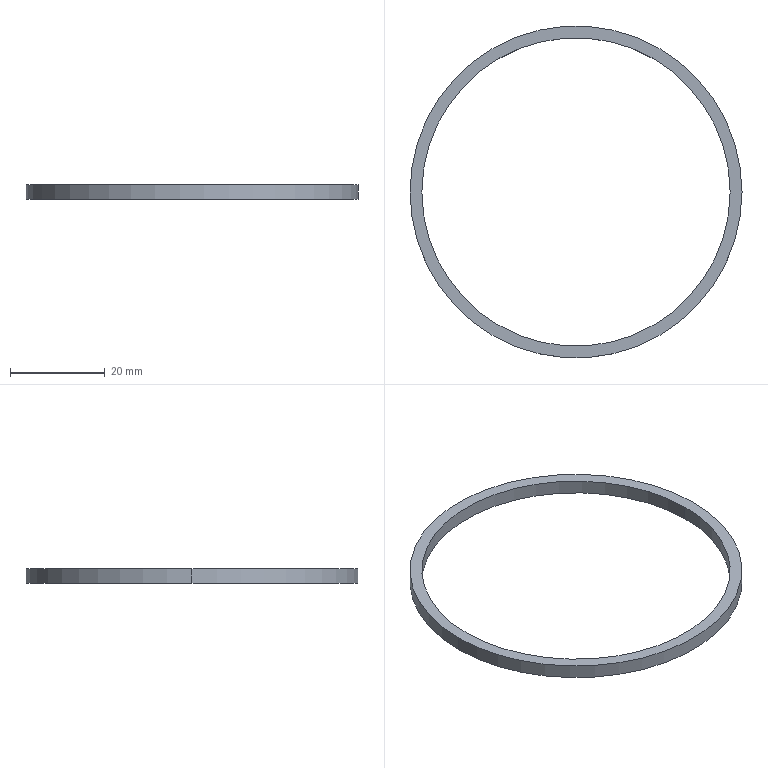Part | SolidWorks | features Extrusion 1 | 1 solid | 6 faces | box 70 x 70 x 3 mm | volume 1590 mm3 | cylinder 4 | plane 2 | commonest cylinder face diameters 65 x2 70 x2
STEP:
#1=CARTESIAN_POINT('',(-32.5,0.,3.));
#2=VERTEX_POINT('',#1);
#3=CARTESIAN_POINT('',(32.5,0.,3.));
#4=VERTEX_POINT('',#3);
#5=CARTESIAN_POINT('',(0.,0.,3.));
#6=DIRECTION('',(0.,0.,1.));
#7=DIRECTION('',(1.,0.,0.));
#8=AXIS2_PLACEMENT_3D('',#5,#6,#7);
#9=CIRCLE('',#8,32.5);
#10=EDGE_CURVE('',#2,#4,#9,.T.);
#11=ORIENTED_EDGE('',*,*,#10,.T.);
#12=CARTESIAN_POINT('',(32.5,0.,0.));
#13=VERTEX_POINT('',#12);
#14=CARTESIAN_POINT('',(32.5,0.,3.));
#15=DIRECTION('',(0.,0.,-1.));
#16=VECTOR('',#15,1000.);
#17=LINE('',#14,#16);
#18=EDGE_CURVE('',#4,#13,#17,.T.);
#19=ORIENTED_EDGE('',*,*,#18,.T.);
#20=CARTESIAN_POINT('',(-32.5,0.,0.));
#21=VERTEX_POINT('',#20);
#22=CARTESIAN_POINT('',(0.,0.,0.));
#23=DIRECTION('',(0.,0.,1.));
#24=DIRECTION('',(1.,0.,0.));
#25=AXIS2_PLACEMENT_3D('',#22,#23,#24);
#26=CIRCLE('',#25,32.5);
#27=EDGE_CURVE('',#21,#13,#26,.T.);
#28=ORIENTED_EDGE('',*,*,#27,.F.);
#29=CARTESIAN_POINT('',(-32.5,0.,3.));
#30=DIRECTION('',(0.,0.,-1.));
#31=VECTOR('',#30,1000.);
#32=LINE('',#29,#31);
#33=EDGE_CURVE('',#2,#21,#32,.T.);
#34=ORIENTED_EDGE('',*,*,#33,.F.);
#35=EDGE_LOOP('',(#11,#19,#28,#34));
#36=FACE_OUTER_BOUND('',#35,.T.);
#37=CARTESIAN_POINT('',(0.,0.,3.));
#38=DIRECTION('',(0.,0.,-1.));
#39=DIRECTION('',(-1.,0.,0.));
#40=AXIS2_PLACEMENT_3D('',#37,#38,#39);
#41=CYLINDRICAL_SURFACE('',#40,32.5);
#42=ADVANCED_FACE('',(#36),#41,.F.);
#43=CARTESIAN_POINT('',(35.,0.,3.));
#44=VERTEX_POINT('',#43);
#45=CARTESIAN_POINT('',(-35.,0.,3.));
#46=VERTEX_POINT('',#45);
#47=CARTESIAN_POINT('',(0.,0.,3.));
#48=DIRECTION('',(0.,0.,1.));
#49=DIRECTION('',(1.,0.,0.));
#50=AXIS2_PLACEMENT_3D('',#47,#48,#49);
#51=CIRCLE('',#50,35.);
#52=EDGE_CURVE('',#44,#46,#51,.T.);
#53=ORIENTED_EDGE('',*,*,#52,.F.);
#54=CARTESIAN_POINT('',(35.,0.,0.));
#55=VERTEX_POINT('',#54);
#56=CARTESIAN_POINT('',(35.,0.,3.));
#57=DIRECTION('',(0.,0.,-1.));
#58=VECTOR('',#57,1000.);
#59=LINE('',#56,#58);
#60=EDGE_CURVE('',#44,#55,#59,.T.);
#61=ORIENTED_EDGE('',*,*,#60,.T.);
#62=CARTESIAN_POINT('',(-35.,0.,0.));
#63=VERTEX_POINT('',#62);
#64=CARTESIAN_POINT('',(0.,0.,0.));
#65=DIRECTION('',(0.,0.,1.));
#66=DIRECTION('',(1.,0.,0.));
#67=AXIS2_PLACEMENT_3D('',#64,#65,#66);
#68=CIRCLE('',#67,35.);
#69=EDGE_CURVE('',#55,#63,#68,.T.);
#70=ORIENTED_EDGE('',*,*,#69,.T.);
#71=CARTESIAN_POINT('',(-35.,0.,3.));
#72=DIRECTION('',(0.,0.,-1.));
#73=VECTOR('',#72,1000.);
#74=LINE('',#71,#73);
#75=EDGE_CURVE('',#46,#63,#74,.T.);
#76=ORIENTED_EDGE('',*,*,#75,.F.);
#77=EDGE_LOOP('',(#53,#61,#70,#76));
#78=FACE_OUTER_BOUND('',#77,.T.);
#79=CARTESIAN_POINT('',(0.,0.,3.));
#80=DIRECTION('',(0.,0.,-1.));
#81=DIRECTION('',(-1.,0.,0.));
#82=AXIS2_PLACEMENT_3D('',#79,#80,#81);
#83=CYLINDRICAL_SURFACE('',#82,35.);
#84=ADVANCED_FACE('',(#78),#83,.T.);
#85=CARTESIAN_POINT('',(0.,0.,3.));
#86=DIRECTION('',(0.,0.,1.));
#87=DIRECTION('',(1.,0.,0.));
#88=AXIS2_PLACEMENT_3D('',#85,#86,#87);
#89=CIRCLE('',#88,35.);
#90=EDGE_CURVE('',#46,#44,#89,.T.);
#91=ORIENTED_EDGE('',*,*,#90,.T.);
#92=ORIENTED_EDGE('',*,*,#52,.T.);
#93=EDGE_LOOP('',(#91,#92));
#94=FACE_OUTER_BOUND('',#93,.T.);
#95=ORIENTED_EDGE('',*,*,#10,.F.);
#96=CARTESIAN_POINT('',(0.,0.,3.));
#97=DIRECTION('',(0.,0.,1.));
#98=DIRECTION('',(1.,0.,0.));
#99=AXIS2_PLACEMENT_3D('',#96,#97,#98);
#100=CIRCLE('',#99,32.5);
#101=EDGE_CURVE('',#4,#2,#100,.T.);
#102=ORIENTED_EDGE('',*,*,#101,.F.);
#103=EDGE_LOOP('',(#95,#102));
#104=FACE_BOUND('',#103,.T.);
#105=CARTESIAN_POINT('',(0.,0.,3.));
#106=DIRECTION('',(0.,0.,1.));
#107=DIRECTION('',(1.,0.,0.));
#108=AXIS2_PLACEMENT_3D('',#105,#106,#107);
#109=PLANE('',#108);
#110=ADVANCED_FACE('',(#94,#104),#109,.T.);
#111=CARTESIAN_POINT('',(0.,0.,0.));
#112=DIRECTION('',(0.,0.,1.));
#113=DIRECTION('',(1.,0.,0.));
#114=AXIS2_PLACEMENT_3D('',#111,#112,#113);
#115=CIRCLE('',#114,35.);
#116=EDGE_CURVE('',#63,#55,#115,.T.);
#117=ORIENTED_EDGE('',*,*,#116,.F.);
#118=ORIENTED_EDGE('',*,*,#69,.F.);
#119=EDGE_LOOP('',(#117,#118));
#120=FACE_OUTER_BOUND('',#119,.T.);
#121=ORIENTED_EDGE('',*,*,#27,.T.);
#122=CARTESIAN_POINT('',(0.,0.,0.));
#123=DIRECTION('',(0.,0.,1.));
#124=DIRECTION('',(1.,0.,0.));
#125=AXIS2_PLACEMENT_3D('',#122,#123,#124);
#126=CIRCLE('',#125,32.5);
#127=EDGE_CURVE('',#13,#21,#126,.T.);
#128=ORIENTED_EDGE('',*,*,#127,.T.);
#129=EDGE_LOOP('',(#121,#128));
#130=FACE_BOUND('',#129,.T.);
#131=CARTESIAN_POINT('',(0.,0.,0.));
#132=DIRECTION('',(0.,0.,1.));
#133=DIRECTION('',(1.,0.,0.));
#134=AXIS2_PLACEMENT_3D('',#131,#132,#133);
#135=PLANE('',#134);
#136=ADVANCED_FACE('',(#120,#130),#135,.F.);
#137=ORIENTED_EDGE('',*,*,#60,.F.);
#138=ORIENTED_EDGE('',*,*,#90,.F.);
#139=ORIENTED_EDGE('',*,*,#75,.T.);
#140=ORIENTED_EDGE('',*,*,#116,.T.);
#141=EDGE_LOOP('',(#137,#138,#139,#140));
#142=FACE_OUTER_BOUND('',#141,.T.);
#143=CARTESIAN_POINT('',(0.,0.,3.));
#144=DIRECTION('',(0.,0.,-1.));
#145=DIRECTION('',(-1.,0.,0.));
#146=AXIS2_PLACEMENT_3D('',#143,#144,#145);
#147=CYLINDRICAL_SURFACE('',#146,35.);
#148=ADVANCED_FACE('',(#142),#147,.T.);
#149=ORIENTED_EDGE('',*,*,#18,.F.);
#150=ORIENTED_EDGE('',*,*,#101,.T.);
#151=ORIENTED_EDGE('',*,*,#33,.T.);
#152=ORIENTED_EDGE('',*,*,#127,.F.);
#153=EDGE_LOOP('',(#149,#150,#151,#152));
#154=FACE_OUTER_BOUND('',#153,.T.);
#155=CARTESIAN_POINT('',(0.,0.,3.));
#156=DIRECTION('',(0.,0.,-1.));
#157=DIRECTION('',(-1.,0.,0.));
#158=AXIS2_PLACEMENT_3D('',#155,#156,#157);
#159=CYLINDRICAL_SURFACE('',#158,32.5);
#160=ADVANCED_FACE('',(#154),#159,.F.);
#161=CLOSED_SHELL('',(#42,#84,#110,#136,#148,#160));
#162=MANIFOLD_SOLID_BREP('',#161);
#163=CARTESIAN_POINT('',(0.,0.,0.));
#164=DIRECTION('',(0.,0.,1.));
#165=DIRECTION('',(1.,0.,0.));
#166=AXIS2_PLACEMENT_3D('',#163,#164,#165);
#167=(LENGTH_UNIT()NAMED_UNIT(*)SI_UNIT(.MILLI.,.METRE.));
#168=UNCERTAINTY_MEASURE_WITH_UNIT(LENGTH_MEASURE(0.00001),#167,'','');
#169=(NAMED_UNIT(*)PLANE_ANGLE_UNIT()SI_UNIT($,.RADIAN.));
#170=(NAMED_UNIT(*)SI_UNIT($,.STERADIAN.)SOLID_ANGLE_UNIT());
#171=(GEOMETRIC_REPRESENTATION_CONTEXT(3)GLOBAL_UNCERTAINTY_ASSIGNED_CONTEXT((#168))GLOBAL_UNIT_ASSIGNED_CONTEXT((#167,#169,#170))REPRESENTATION_CONTEXT('',''));
#172=ADVANCED_BREP_SHAPE_REPRESENTATION('',(#162,#166),#171);